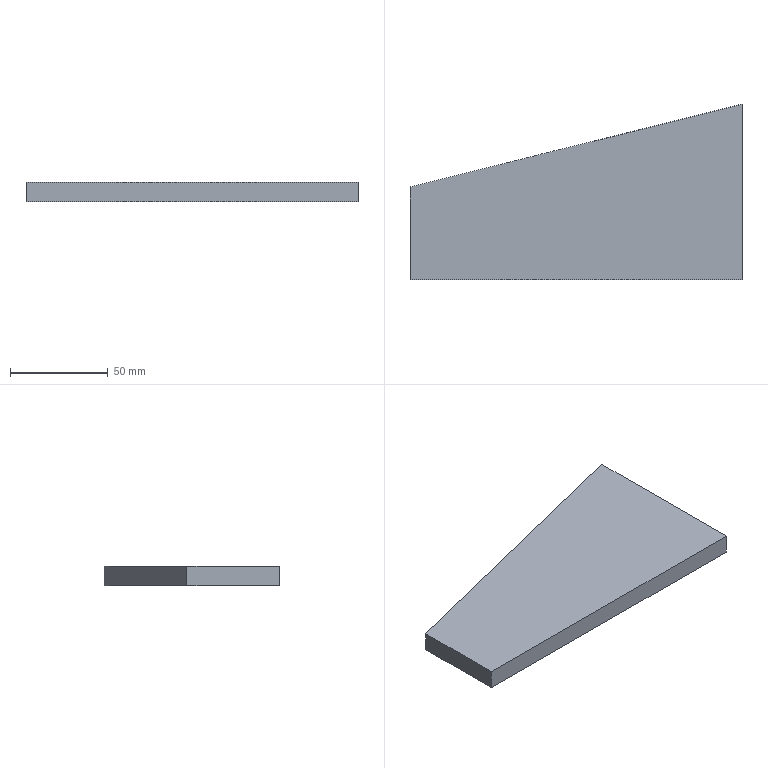Part | STEP file | 001-004-Feeding mechanism shaft slideway side plate | 1 solid | 6 faces | box 170 x 90 x 10 mm | volume 116972 mm3 | plane 6
STEP:
#1=CARTESIAN_POINT('',(0.,0.,0.));
#2=DIRECTION('',(0.,0.,1.));
#3=DIRECTION('',(1.,0.,0.));
#4=AXIS2_PLACEMENT_3D('',#1,#2,#3);
#5=CARTESIAN_POINT('',(85.,-45.,0.));
#6=VERTEX_POINT('',#5);
#7=CARTESIAN_POINT('',(85.,45.,0.));
#8=VERTEX_POINT('',#7);
#9=CARTESIAN_POINT('',(85.,-45.,0.));
#10=DIRECTION('',(0.,1.,0.));
#11=VECTOR('',#10,1.);
#12=LINE('',#9,#11);
#13=CARTESIAN_POINT('',(85.,-45.,10.));
#14=DIRECTION('',(-1.,0.,0.));
#15=DIRECTION('',(0.,0.,1.));
#16=AXIS2_PLACEMENT_3D('',#13,#14,#15);
#17=PLANE('',#16);
#18=CARTESIAN_POINT('',(-10.,0.));
#19=DIRECTION('',(0.,1.));
#20=VECTOR('',#19,1.);
#21=LINE('',#18,#20);
#22=(GEOMETRIC_REPRESENTATION_CONTEXT(2)PARAMETRIC_REPRESENTATION_CONTEXT()REPRESENTATION_CONTEXT('',''));
#23=DEFINITIONAL_REPRESENTATION('',(#21),#22);
#24=PCURVE('',#17,#23);
#25=CARTESIAN_POINT('',(0.,0.,0.));
#26=DIRECTION('',(0.,0.,-1.));
#27=DIRECTION('',(-1.,0.,0.));
#28=AXIS2_PLACEMENT_3D('',#25,#26,#27);
#29=PLANE('',#28);
#30=CARTESIAN_POINT('',(-85.,-45.));
#31=DIRECTION('',(0.,1.));
#32=VECTOR('',#31,1.);
#33=LINE('',#30,#32);
#34=(GEOMETRIC_REPRESENTATION_CONTEXT(2)PARAMETRIC_REPRESENTATION_CONTEXT()REPRESENTATION_CONTEXT('',''));
#35=DEFINITIONAL_REPRESENTATION('',(#33),#34);
#36=PCURVE('',#29,#35);
#37=SURFACE_CURVE('',#12,(#24,#36),.PCURVE_S1.);
#38=EDGE_CURVE('',#6,#8,#37,.T.);
#39=ORIENTED_EDGE('',*,*,#38,.T.);
#40=CARTESIAN_POINT('',(85.,45.,10.));
#41=VERTEX_POINT('',#40);
#42=CARTESIAN_POINT('',(85.,45.,10.));
#43=DIRECTION('',(0.,0.,-1.));
#44=VECTOR('',#43,1.);
#45=LINE('',#42,#44);
#46=CARTESIAN_POINT('',(0.,90.));
#47=DIRECTION('',(-1.,0.));
#48=VECTOR('',#47,1.);
#49=LINE('',#46,#48);
#50=(GEOMETRIC_REPRESENTATION_CONTEXT(2)PARAMETRIC_REPRESENTATION_CONTEXT()REPRESENTATION_CONTEXT('',''));
#51=DEFINITIONAL_REPRESENTATION('',(#49),#50);
#52=PCURVE('',#17,#51);
#53=CARTESIAN_POINT('',(85.,45.,0.));
#54=DIRECTION('',(0.2419,-0.9703,0.));
#55=DIRECTION('',(0.9703,0.2419,0.));
#56=AXIS2_PLACEMENT_3D('',#53,#54,#55);
#57=PLANE('',#56);
#58=CARTESIAN_POINT('',(0.,10.));
#59=DIRECTION('',(0.,-1.));
#60=VECTOR('',#59,1.);
#61=LINE('',#58,#60);
#62=(GEOMETRIC_REPRESENTATION_CONTEXT(2)PARAMETRIC_REPRESENTATION_CONTEXT()REPRESENTATION_CONTEXT('',''));
#63=DEFINITIONAL_REPRESENTATION('',(#61),#62);
#64=PCURVE('',#57,#63);
#65=SURFACE_CURVE('',#45,(#52,#64),.PCURVE_S1.);
#66=EDGE_CURVE('',#41,#8,#65,.T.);
#67=ORIENTED_EDGE('',*,*,#66,.F.);
#68=CARTESIAN_POINT('',(85.,-45.,10.));
#69=VERTEX_POINT('',#68);
#70=CARTESIAN_POINT('',(85.,-45.,10.));
#71=DIRECTION('',(0.,1.,0.));
#72=VECTOR('',#71,1.);
#73=LINE('',#70,#72);
#74=CARTESIAN_POINT('',(0.,0.));
#75=DIRECTION('',(0.,1.));
#76=VECTOR('',#75,1.);
#77=LINE('',#74,#76);
#78=(GEOMETRIC_REPRESENTATION_CONTEXT(2)PARAMETRIC_REPRESENTATION_CONTEXT()REPRESENTATION_CONTEXT('',''));
#79=DEFINITIONAL_REPRESENTATION('',(#77),#78);
#80=PCURVE('',#17,#79);
#81=CARTESIAN_POINT('',(0.,0.,10.));
#82=DIRECTION('',(0.,0.,-1.));
#83=DIRECTION('',(-1.,0.,0.));
#84=AXIS2_PLACEMENT_3D('',#81,#82,#83);
#85=PLANE('',#84);
#86=CARTESIAN_POINT('',(-85.,-45.));
#87=DIRECTION('',(0.,1.));
#88=VECTOR('',#87,1.);
#89=LINE('',#86,#88);
#90=(GEOMETRIC_REPRESENTATION_CONTEXT(2)PARAMETRIC_REPRESENTATION_CONTEXT()REPRESENTATION_CONTEXT('',''));
#91=DEFINITIONAL_REPRESENTATION('',(#89),#90);
#92=PCURVE('',#85,#91);
#93=SURFACE_CURVE('',#73,(#80,#92),.PCURVE_S1.);
#94=EDGE_CURVE('',#69,#41,#93,.T.);
#95=ORIENTED_EDGE('',*,*,#94,.F.);
#96=CARTESIAN_POINT('',(85.,-45.,10.));
#97=DIRECTION('',(0.,0.,-1.));
#98=VECTOR('',#97,1.);
#99=LINE('',#96,#98);
#100=CARTESIAN_POINT('',(0.,0.));
#101=DIRECTION('',(-1.,0.));
#102=VECTOR('',#101,1.);
#103=LINE('',#100,#102);
#104=(GEOMETRIC_REPRESENTATION_CONTEXT(2)PARAMETRIC_REPRESENTATION_CONTEXT()REPRESENTATION_CONTEXT('',''));
#105=DEFINITIONAL_REPRESENTATION('',(#103),#104);
#106=PCURVE('',#17,#105);
#107=CARTESIAN_POINT('',(-85.,-45.,10.));
#108=DIRECTION('',(0.,1.,0.));
#109=DIRECTION('',(0.,0.,1.));
#110=AXIS2_PLACEMENT_3D('',#107,#108,#109);
#111=PLANE('',#110);
#112=CARTESIAN_POINT('',(0.,170.));
#113=DIRECTION('',(-1.,0.));
#114=VECTOR('',#113,1.);
#115=LINE('',#112,#114);
#116=(GEOMETRIC_REPRESENTATION_CONTEXT(2)PARAMETRIC_REPRESENTATION_CONTEXT()REPRESENTATION_CONTEXT('',''));
#117=DEFINITIONAL_REPRESENTATION('',(#115),#116);
#118=PCURVE('',#111,#117);
#119=SURFACE_CURVE('',#99,(#106,#118),.PCURVE_S1.);
#120=EDGE_CURVE('',#69,#6,#119,.T.);
#121=ORIENTED_EDGE('',*,*,#120,.T.);
#122=EDGE_LOOP('',(#39,#67,#95,#121));
#123=FACE_BOUND('',#122,.T.);
#124=ADVANCED_FACE('',(#123),#17,.F.);
#125=CARTESIAN_POINT('',(-85.,2.614,10.));
#126=VERTEX_POINT('',#125);
#127=CARTESIAN_POINT('',(-85.,-45.,10.));
#128=VERTEX_POINT('',#127);
#129=CARTESIAN_POINT('',(-85.,-45.,10.));
#130=DIRECTION('',(0.,-1.,0.));
#131=VECTOR('',#130,1.);
#132=LINE('',#129,#131);
#133=CARTESIAN_POINT('',(-85.,-45.,10.));
#134=DIRECTION('',(1.,0.,0.));
#135=DIRECTION('',(0.,0.,-1.));
#136=AXIS2_PLACEMENT_3D('',#133,#134,#135);
#137=PLANE('',#136);
#138=CARTESIAN_POINT('',(0.,0.));
#139=DIRECTION('',(0.,-1.));
#140=VECTOR('',#139,1.);
#141=LINE('',#138,#140);
#142=(GEOMETRIC_REPRESENTATION_CONTEXT(2)PARAMETRIC_REPRESENTATION_CONTEXT()REPRESENTATION_CONTEXT('',''));
#143=DEFINITIONAL_REPRESENTATION('',(#141),#142);
#144=PCURVE('',#137,#143);
#145=CARTESIAN_POINT('',(85.,-45.));
#146=DIRECTION('',(0.,-1.));
#147=VECTOR('',#146,1.);
#148=LINE('',#145,#147);
#149=(GEOMETRIC_REPRESENTATION_CONTEXT(2)PARAMETRIC_REPRESENTATION_CONTEXT()REPRESENTATION_CONTEXT('',''));
#150=DEFINITIONAL_REPRESENTATION('',(#148),#149);
#151=PCURVE('',#85,#150);
#152=SURFACE_CURVE('',#132,(#144,#151),.PCURVE_S1.);
#153=EDGE_CURVE('',#126,#128,#152,.T.);
#154=ORIENTED_EDGE('',*,*,#153,.F.);
#155=CARTESIAN_POINT('',(-85.,2.614,0.));
#156=VERTEX_POINT('',#155);
#157=CARTESIAN_POINT('',(-85.,2.614,0.));
#158=DIRECTION('',(0.,0.,1.));
#159=VECTOR('',#158,1.);
#160=LINE('',#157,#159);
#161=CARTESIAN_POINT('',(10.,47.614));
#162=DIRECTION('',(-1.,0.));
#163=VECTOR('',#162,1.);
#164=LINE('',#161,#163);
#165=(GEOMETRIC_REPRESENTATION_CONTEXT(2)PARAMETRIC_REPRESENTATION_CONTEXT()REPRESENTATION_CONTEXT('',''));
#166=DEFINITIONAL_REPRESENTATION('',(#164),#165);
#167=PCURVE('',#137,#166);
#168=CARTESIAN_POINT('',(-175.204,0.));
#169=DIRECTION('',(0.,1.));
#170=VECTOR('',#169,1.);
#171=LINE('',#168,#170);
#172=(GEOMETRIC_REPRESENTATION_CONTEXT(2)PARAMETRIC_REPRESENTATION_CONTEXT()REPRESENTATION_CONTEXT('',''));
#173=DEFINITIONAL_REPRESENTATION('',(#171),#172);
#174=PCURVE('',#57,#173);
#175=SURFACE_CURVE('',#160,(#167,#174),.PCURVE_S1.);
#176=EDGE_CURVE('',#156,#126,#175,.T.);
#177=ORIENTED_EDGE('',*,*,#176,.F.);
#178=CARTESIAN_POINT('',(-85.,-45.,0.));
#179=VERTEX_POINT('',#178);
#180=CARTESIAN_POINT('',(-85.,-45.,0.));
#181=DIRECTION('',(0.,-1.,0.));
#182=VECTOR('',#181,1.);
#183=LINE('',#180,#182);
#184=CARTESIAN_POINT('',(10.,0.));
#185=DIRECTION('',(0.,-1.));
#186=VECTOR('',#185,1.);
#187=LINE('',#184,#186);
#188=(GEOMETRIC_REPRESENTATION_CONTEXT(2)PARAMETRIC_REPRESENTATION_CONTEXT()REPRESENTATION_CONTEXT('',''));
#189=DEFINITIONAL_REPRESENTATION('',(#187),#188);
#190=PCURVE('',#137,#189);
#191=CARTESIAN_POINT('',(85.,-45.));
#192=DIRECTION('',(0.,-1.));
#193=VECTOR('',#192,1.);
#194=LINE('',#191,#193);
#195=(GEOMETRIC_REPRESENTATION_CONTEXT(2)PARAMETRIC_REPRESENTATION_CONTEXT()REPRESENTATION_CONTEXT('',''));
#196=DEFINITIONAL_REPRESENTATION('',(#194),#195);
#197=PCURVE('',#29,#196);
#198=SURFACE_CURVE('',#183,(#190,#197),.PCURVE_S1.);
#199=EDGE_CURVE('',#156,#179,#198,.T.);
#200=ORIENTED_EDGE('',*,*,#199,.T.);
#201=CARTESIAN_POINT('',(-85.,-45.,10.));
#202=DIRECTION('',(0.,0.,-1.));
#203=VECTOR('',#202,1.);
#204=LINE('',#201,#203);
#205=CARTESIAN_POINT('',(0.,0.));
#206=DIRECTION('',(1.,0.));
#207=VECTOR('',#206,1.);
#208=LINE('',#205,#207);
#209=(GEOMETRIC_REPRESENTATION_CONTEXT(2)PARAMETRIC_REPRESENTATION_CONTEXT()REPRESENTATION_CONTEXT('',''));
#210=DEFINITIONAL_REPRESENTATION('',(#208),#209);
#211=PCURVE('',#137,#210);
#212=CARTESIAN_POINT('',(0.,0.));
#213=DIRECTION('',(-1.,0.));
#214=VECTOR('',#213,1.);
#215=LINE('',#212,#214);
#216=(GEOMETRIC_REPRESENTATION_CONTEXT(2)PARAMETRIC_REPRESENTATION_CONTEXT()REPRESENTATION_CONTEXT('',''));
#217=DEFINITIONAL_REPRESENTATION('',(#215),#216);
#218=PCURVE('',#111,#217);
#219=SURFACE_CURVE('',#204,(#211,#218),.PCURVE_S1.);
#220=EDGE_CURVE('',#128,#179,#219,.T.);
#221=ORIENTED_EDGE('',*,*,#220,.F.);
#222=EDGE_LOOP('',(#154,#177,#200,#221));
#223=FACE_BOUND('',#222,.T.);
#224=ADVANCED_FACE('',(#223),#137,.F.);
#225=CARTESIAN_POINT('',(-85.,-45.,0.));
#226=DIRECTION('',(1.,0.,0.));
#227=VECTOR('',#226,1.);
#228=LINE('',#225,#227);
#229=CARTESIAN_POINT('',(-10.,0.));
#230=DIRECTION('',(0.,1.));
#231=VECTOR('',#230,1.);
#232=LINE('',#229,#231);
#233=(GEOMETRIC_REPRESENTATION_CONTEXT(2)PARAMETRIC_REPRESENTATION_CONTEXT()REPRESENTATION_CONTEXT('',''));
#234=DEFINITIONAL_REPRESENTATION('',(#232),#233);
#235=PCURVE('',#111,#234);
#236=CARTESIAN_POINT('',(85.,-45.));
#237=DIRECTION('',(-1.,0.));
#238=VECTOR('',#237,1.);
#239=LINE('',#236,#238);
#240=(GEOMETRIC_REPRESENTATION_CONTEXT(2)PARAMETRIC_REPRESENTATION_CONTEXT()REPRESENTATION_CONTEXT('',''));
#241=DEFINITIONAL_REPRESENTATION('',(#239),#240);
#242=PCURVE('',#29,#241);
#243=SURFACE_CURVE('',#228,(#235,#242),.PCURVE_S1.);
#244=EDGE_CURVE('',#179,#6,#243,.T.);
#245=ORIENTED_EDGE('',*,*,#244,.T.);
#246=ORIENTED_EDGE('',*,*,#120,.F.);
#247=CARTESIAN_POINT('',(-85.,-45.,10.));
#248=DIRECTION('',(1.,0.,0.));
#249=VECTOR('',#248,1.);
#250=LINE('',#247,#249);
#251=CARTESIAN_POINT('',(0.,0.));
#252=DIRECTION('',(0.,1.));
#253=VECTOR('',#252,1.);
#254=LINE('',#251,#253);
#255=(GEOMETRIC_REPRESENTATION_CONTEXT(2)PARAMETRIC_REPRESENTATION_CONTEXT()REPRESENTATION_CONTEXT('',''));
#256=DEFINITIONAL_REPRESENTATION('',(#254),#255);
#257=PCURVE('',#111,#256);
#258=CARTESIAN_POINT('',(85.,-45.));
#259=DIRECTION('',(-1.,0.));
#260=VECTOR('',#259,1.);
#261=LINE('',#258,#260);
#262=(GEOMETRIC_REPRESENTATION_CONTEXT(2)PARAMETRIC_REPRESENTATION_CONTEXT()REPRESENTATION_CONTEXT('',''));
#263=DEFINITIONAL_REPRESENTATION('',(#261),#262);
#264=PCURVE('',#85,#263);
#265=SURFACE_CURVE('',#250,(#257,#264),.PCURVE_S1.);
#266=EDGE_CURVE('',#128,#69,#265,.T.);
#267=ORIENTED_EDGE('',*,*,#266,.F.);
#268=ORIENTED_EDGE('',*,*,#220,.T.);
#269=EDGE_LOOP('',(#245,#246,#267,#268));
#270=FACE_BOUND('',#269,.T.);
#271=ADVANCED_FACE('',(#270),#111,.F.);
#272=ORIENTED_EDGE('',*,*,#94,.T.);
#273=CARTESIAN_POINT('',(85.,45.,10.));
#274=DIRECTION('',(0.9703,0.2419,0.));
#275=VECTOR('',#274,1.);
#276=LINE('',#273,#275);
#277=CARTESIAN_POINT('',(-85.,45.));
#278=DIRECTION('',(-0.9703,0.2419));
#279=VECTOR('',#278,1.);
#280=LINE('',#277,#279);
#281=(GEOMETRIC_REPRESENTATION_CONTEXT(2)PARAMETRIC_REPRESENTATION_CONTEXT()REPRESENTATION_CONTEXT('',''));
#282=DEFINITIONAL_REPRESENTATION('',(#280),#281);
#283=PCURVE('',#85,#282);
#284=CARTESIAN_POINT('',(0.,10.));
#285=DIRECTION('',(1.,0.));
#286=VECTOR('',#285,1.);
#287=LINE('',#284,#286);
#288=(GEOMETRIC_REPRESENTATION_CONTEXT(2)PARAMETRIC_REPRESENTATION_CONTEXT()REPRESENTATION_CONTEXT('',''));
#289=DEFINITIONAL_REPRESENTATION('',(#287),#288);
#290=PCURVE('',#57,#289);
#291=SURFACE_CURVE('',#276,(#283,#290),.PCURVE_S1.);
#292=EDGE_CURVE('',#126,#41,#291,.T.);
#293=ORIENTED_EDGE('',*,*,#292,.F.);
#294=ORIENTED_EDGE('',*,*,#153,.T.);
#295=ORIENTED_EDGE('',*,*,#266,.T.);
#296=EDGE_LOOP('',(#272,#293,#294,#295));
#297=FACE_BOUND('',#296,.T.);
#298=ADVANCED_FACE('',(#297),#85,.F.);
#299=CARTESIAN_POINT('',(85.,45.,0.));
#300=DIRECTION('',(0.9703,0.2419,0.));
#301=VECTOR('',#300,1.);
#302=LINE('',#299,#301);
#303=CARTESIAN_POINT('',(-85.,45.));
#304=DIRECTION('',(-0.9703,0.2419));
#305=VECTOR('',#304,1.);
#306=LINE('',#303,#305);
#307=(GEOMETRIC_REPRESENTATION_CONTEXT(2)PARAMETRIC_REPRESENTATION_CONTEXT()REPRESENTATION_CONTEXT('',''));
#308=DEFINITIONAL_REPRESENTATION('',(#306),#307);
#309=PCURVE('',#29,#308);
#310=CARTESIAN_POINT('',(0.,0.));
#311=DIRECTION('',(1.,0.));
#312=VECTOR('',#311,1.);
#313=LINE('',#310,#312);
#314=(GEOMETRIC_REPRESENTATION_CONTEXT(2)PARAMETRIC_REPRESENTATION_CONTEXT()REPRESENTATION_CONTEXT('',''));
#315=DEFINITIONAL_REPRESENTATION('',(#313),#314);
#316=PCURVE('',#57,#315);
#317=SURFACE_CURVE('',#302,(#309,#316),.PCURVE_S1.);
#318=EDGE_CURVE('',#156,#8,#317,.T.);
#319=ORIENTED_EDGE('',*,*,#318,.T.);
#320=ORIENTED_EDGE('',*,*,#38,.F.);
#321=ORIENTED_EDGE('',*,*,#244,.F.);
#322=ORIENTED_EDGE('',*,*,#199,.F.);
#323=EDGE_LOOP('',(#319,#320,#321,#322));
#324=FACE_BOUND('',#323,.T.);
#325=ADVANCED_FACE('',(#324),#29,.T.);
#326=ORIENTED_EDGE('',*,*,#292,.T.);
#327=ORIENTED_EDGE('',*,*,#66,.T.);
#328=ORIENTED_EDGE('',*,*,#318,.F.);
#329=ORIENTED_EDGE('',*,*,#176,.T.);
#330=EDGE_LOOP('',(#326,#327,#328,#329));
#331=FACE_BOUND('',#330,.T.);
#332=ADVANCED_FACE('',(#331),#57,.F.);
#333=CLOSED_SHELL('',(#124,#224,#271,#298,#325,#332));
#334=MANIFOLD_SOLID_BREP('',#333);
#335=(LENGTH_UNIT()NAMED_UNIT(*)SI_UNIT(.MILLI.,.METRE.));
#336=UNCERTAINTY_MEASURE_WITH_UNIT(LENGTH_MEASURE(0.0000001),#335,'','');
#337=(NAMED_UNIT(*)PLANE_ANGLE_UNIT()SI_UNIT($,.RADIAN.));
#338=(NAMED_UNIT(*)SI_UNIT($,.STERADIAN.)SOLID_ANGLE_UNIT());
#339=(GEOMETRIC_REPRESENTATION_CONTEXT(3)GLOBAL_UNCERTAINTY_ASSIGNED_CONTEXT((#336))GLOBAL_UNIT_ASSIGNED_CONTEXT((#335,#337,#338))REPRESENTATION_CONTEXT('',''));
#340=ADVANCED_BREP_SHAPE_REPRESENTATION('',(#4,#334),#339);